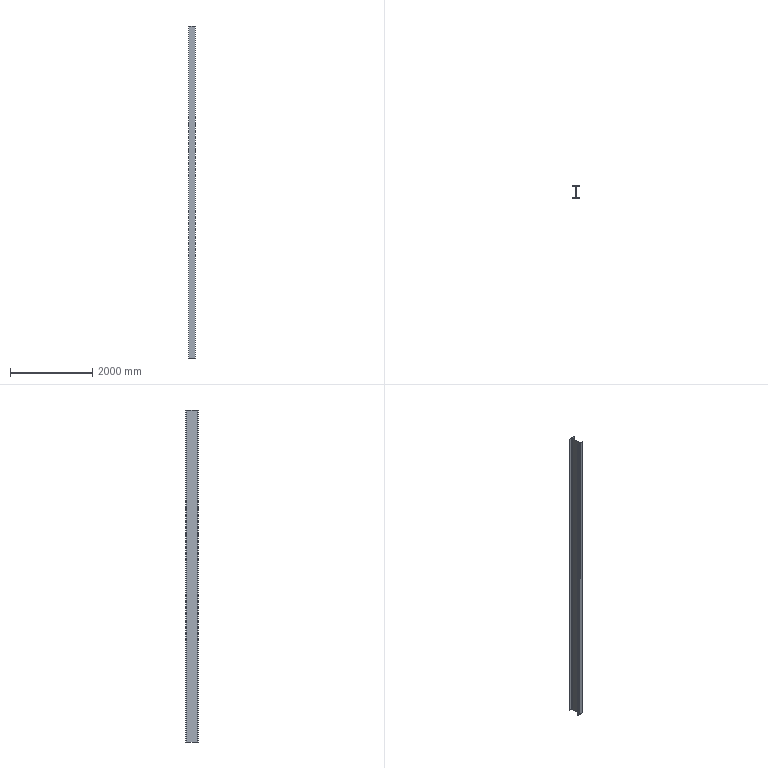Part | SolidWorks | features Extrusion 1 | 1 solid | 18 faces | box 150 x 300 x 8060 mm | volume 37705251 mm3 | plane 14 | cylinder 4 | commonest cylinder face diameters 26 x4
STEP:
#1=CARTESIAN_POINT('',(-75.,9.,0.));
#2=VERTEX_POINT('',#1);
#3=CARTESIAN_POINT('',(-75.,0.,0.));
#4=VERTEX_POINT('',#3);
#5=CARTESIAN_POINT('',(-75.,0.,0.));
#6=DIRECTION('',(0.,-1.,0.));
#7=VECTOR('',#6,1000.);
#8=LINE('',#5,#7);
#9=EDGE_CURVE('',#2,#4,#8,.T.);
#10=ORIENTED_EDGE('',*,*,#9,.T.);
#11=CARTESIAN_POINT('',(-75.,0.,8060.));
#12=VERTEX_POINT('',#11);
#13=CARTESIAN_POINT('',(-75.,0.,8060.));
#14=DIRECTION('',(0.,0.,-1.));
#15=VECTOR('',#14,1000.);
#16=LINE('',#13,#15);
#17=EDGE_CURVE('',#12,#4,#16,.T.);
#18=ORIENTED_EDGE('',*,*,#17,.F.);
#19=CARTESIAN_POINT('',(-75.,9.,8060.));
#20=VERTEX_POINT('',#19);
#21=CARTESIAN_POINT('',(-75.,0.,8060.));
#22=DIRECTION('',(0.,-1.,0.));
#23=VECTOR('',#22,1000.);
#24=LINE('',#21,#23);
#25=EDGE_CURVE('',#20,#12,#24,.T.);
#26=ORIENTED_EDGE('',*,*,#25,.F.);
#27=CARTESIAN_POINT('',(-75.,9.,8060.));
#28=DIRECTION('',(0.,0.,-1.));
#29=VECTOR('',#28,1000.);
#30=LINE('',#27,#29);
#31=EDGE_CURVE('',#20,#2,#30,.T.);
#32=ORIENTED_EDGE('',*,*,#31,.T.);
#33=EDGE_LOOP('',(#10,#18,#26,#32));
#34=FACE_OUTER_BOUND('',#33,.T.);
#35=CARTESIAN_POINT('',(-75.,0.,8060.));
#36=DIRECTION('',(1.,0.,0.));
#37=DIRECTION('',(0.,0.,-1.));
#38=AXIS2_PLACEMENT_3D('',#35,#36,#37);
#39=PLANE('',#38);
#40=ADVANCED_FACE('',(#34),#39,.F.);
#41=CARTESIAN_POINT('',(75.,0.,0.));
#42=VERTEX_POINT('',#41);
#43=CARTESIAN_POINT('',(75.,0.,0.));
#44=DIRECTION('',(1.,0.,0.));
#45=VECTOR('',#44,1000.);
#46=LINE('',#43,#45);
#47=EDGE_CURVE('',#4,#42,#46,.T.);
#48=ORIENTED_EDGE('',*,*,#47,.T.);
#49=CARTESIAN_POINT('',(75.,0.,8060.));
#50=VERTEX_POINT('',#49);
#51=CARTESIAN_POINT('',(75.,0.,8060.));
#52=DIRECTION('',(0.,0.,-1.));
#53=VECTOR('',#52,1000.);
#54=LINE('',#51,#53);
#55=EDGE_CURVE('',#50,#42,#54,.T.);
#56=ORIENTED_EDGE('',*,*,#55,.F.);
#57=CARTESIAN_POINT('',(75.,0.,8060.));
#58=DIRECTION('',(1.,0.,0.));
#59=VECTOR('',#58,1000.);
#60=LINE('',#57,#59);
#61=EDGE_CURVE('',#12,#50,#60,.T.);
#62=ORIENTED_EDGE('',*,*,#61,.F.);
#63=ORIENTED_EDGE('',*,*,#17,.T.);
#64=EDGE_LOOP('',(#48,#56,#62,#63));
#65=FACE_OUTER_BOUND('',#64,.T.);
#66=CARTESIAN_POINT('',(75.,0.,8060.));
#67=DIRECTION('',(0.,1.,0.));
#68=DIRECTION('',(-1.,0.,0.));
#69=AXIS2_PLACEMENT_3D('',#66,#67,#68);
#70=PLANE('',#69);
#71=ADVANCED_FACE('',(#65),#70,.F.);
#72=CARTESIAN_POINT('',(75.,9.,0.));
#73=VERTEX_POINT('',#72);
#74=CARTESIAN_POINT('',(75.,0.,0.));
#75=DIRECTION('',(0.,1.,0.));
#76=VECTOR('',#75,1000.);
#77=LINE('',#74,#76);
#78=EDGE_CURVE('',#42,#73,#77,.T.);
#79=ORIENTED_EDGE('',*,*,#78,.T.);
#80=CARTESIAN_POINT('',(75.,9.,8060.));
#81=VERTEX_POINT('',#80);
#82=CARTESIAN_POINT('',(75.,9.,8060.));
#83=DIRECTION('',(0.,0.,-1.));
#84=VECTOR('',#83,1000.);
#85=LINE('',#82,#84);
#86=EDGE_CURVE('',#81,#73,#85,.T.);
#87=ORIENTED_EDGE('',*,*,#86,.F.);
#88=CARTESIAN_POINT('',(75.,0.,8060.));
#89=DIRECTION('',(0.,1.,0.));
#90=VECTOR('',#89,1000.);
#91=LINE('',#88,#90);
#92=EDGE_CURVE('',#50,#81,#91,.T.);
#93=ORIENTED_EDGE('',*,*,#92,.F.);
#94=ORIENTED_EDGE('',*,*,#55,.T.);
#95=EDGE_LOOP('',(#79,#87,#93,#94));
#96=FACE_OUTER_BOUND('',#95,.T.);
#97=CARTESIAN_POINT('',(75.,0.,8060.));
#98=DIRECTION('',(-1.,0.,0.));
#99=DIRECTION('',(0.,0.,1.));
#100=AXIS2_PLACEMENT_3D('',#97,#98,#99);
#101=PLANE('',#100);
#102=ADVANCED_FACE('',(#96),#101,.F.);
#103=CARTESIAN_POINT('',(16.25,9.,0.));
#104=VERTEX_POINT('',#103);
#105=CARTESIAN_POINT('',(75.,9.,0.));
#106=DIRECTION('',(-1.,0.,0.));
#107=VECTOR('',#106,1000.);
#108=LINE('',#105,#107);
#109=EDGE_CURVE('',#73,#104,#108,.T.);
#110=ORIENTED_EDGE('',*,*,#109,.T.);
#111=CARTESIAN_POINT('',(16.25,9.,8060.));
#112=VERTEX_POINT('',#111);
#113=CARTESIAN_POINT('',(16.25,9.,8060.));
#114=DIRECTION('',(0.,0.,-1.));
#115=VECTOR('',#114,1000.);
#116=LINE('',#113,#115);
#117=EDGE_CURVE('',#112,#104,#116,.T.);
#118=ORIENTED_EDGE('',*,*,#117,.F.);
#119=CARTESIAN_POINT('',(75.,9.,8060.));
#120=DIRECTION('',(-1.,0.,0.));
#121=VECTOR('',#120,1000.);
#122=LINE('',#119,#121);
#123=EDGE_CURVE('',#81,#112,#122,.T.);
#124=ORIENTED_EDGE('',*,*,#123,.F.);
#125=ORIENTED_EDGE('',*,*,#86,.T.);
#126=EDGE_LOOP('',(#110,#118,#124,#125));
#127=FACE_OUTER_BOUND('',#126,.T.);
#128=CARTESIAN_POINT('',(75.,9.,8060.));
#129=DIRECTION('',(0.,-1.,0.));
#130=DIRECTION('',(1.,0.,0.));
#131=AXIS2_PLACEMENT_3D('',#128,#129,#130);
#132=PLANE('',#131);
#133=ADVANCED_FACE('',(#127),#132,.F.);
#134=CARTESIAN_POINT('',(3.25,22.,0.));
#135=VERTEX_POINT('',#134);
#136=CARTESIAN_POINT('',(16.25,22.,0.));
#137=DIRECTION('',(0.,0.,-1.));
#138=DIRECTION('',(-1.,0.,0.));
#139=AXIS2_PLACEMENT_3D('',#136,#137,#138);
#140=CIRCLE('',#139,13.);
#141=EDGE_CURVE('',#104,#135,#140,.T.);
#142=ORIENTED_EDGE('',*,*,#141,.T.);
#143=CARTESIAN_POINT('',(3.25,22.,8060.));
#144=VERTEX_POINT('',#143);
#145=CARTESIAN_POINT('',(3.25,22.,8060.));
#146=DIRECTION('',(0.,0.,-1.));
#147=VECTOR('',#146,1000.);
#148=LINE('',#145,#147);
#149=EDGE_CURVE('',#144,#135,#148,.T.);
#150=ORIENTED_EDGE('',*,*,#149,.F.);
#151=CARTESIAN_POINT('',(16.25,22.,8060.));
#152=DIRECTION('',(0.,0.,-1.));
#153=DIRECTION('',(-1.,0.,0.));
#154=AXIS2_PLACEMENT_3D('',#151,#152,#153);
#155=CIRCLE('',#154,13.);
#156=EDGE_CURVE('',#112,#144,#155,.T.);
#157=ORIENTED_EDGE('',*,*,#156,.F.);
#158=ORIENTED_EDGE('',*,*,#117,.T.);
#159=EDGE_LOOP('',(#142,#150,#157,#158));
#160=FACE_OUTER_BOUND('',#159,.T.);
#161=CARTESIAN_POINT('',(16.25,22.,8060.));
#162=DIRECTION('',(0.,0.,-1.));
#163=DIRECTION('',(-1.,0.,0.));
#164=AXIS2_PLACEMENT_3D('',#161,#162,#163);
#165=CYLINDRICAL_SURFACE('',#164,13.);
#166=ADVANCED_FACE('',(#160),#165,.F.);
#167=CARTESIAN_POINT('',(3.25,278.,0.));
#168=VERTEX_POINT('',#167);
#169=CARTESIAN_POINT('',(3.25,22.,0.));
#170=DIRECTION('',(0.,1.,0.));
#171=VECTOR('',#170,1000.);
#172=LINE('',#169,#171);
#173=EDGE_CURVE('',#135,#168,#172,.T.);
#174=ORIENTED_EDGE('',*,*,#173,.T.);
#175=CARTESIAN_POINT('',(3.25,278.,8060.));
#176=VERTEX_POINT('',#175);
#177=CARTESIAN_POINT('',(3.25,278.,8060.));
#178=DIRECTION('',(0.,0.,-1.));
#179=VECTOR('',#178,1000.);
#180=LINE('',#177,#179);
#181=EDGE_CURVE('',#176,#168,#180,.T.);
#182=ORIENTED_EDGE('',*,*,#181,.F.);
#183=CARTESIAN_POINT('',(3.25,22.,8060.));
#184=DIRECTION('',(0.,1.,0.));
#185=VECTOR('',#184,1000.);
#186=LINE('',#183,#185);
#187=EDGE_CURVE('',#144,#176,#186,.T.);
#188=ORIENTED_EDGE('',*,*,#187,.F.);
#189=ORIENTED_EDGE('',*,*,#149,.T.);
#190=EDGE_LOOP('',(#174,#182,#188,#189));
#191=FACE_OUTER_BOUND('',#190,.T.);
#192=CARTESIAN_POINT('',(3.25,22.,8060.));
#193=DIRECTION('',(-1.,0.,0.));
#194=DIRECTION('',(0.,0.,1.));
#195=AXIS2_PLACEMENT_3D('',#192,#193,#194);
#196=PLANE('',#195);
#197=ADVANCED_FACE('',(#191),#196,.F.);
#198=CARTESIAN_POINT('',(16.25,291.,0.));
#199=VERTEX_POINT('',#198);
#200=CARTESIAN_POINT('',(16.25,278.,0.));
#201=DIRECTION('',(0.,0.,-1.));
#202=DIRECTION('',(-1.,0.,0.));
#203=AXIS2_PLACEMENT_3D('',#200,#201,#202);
#204=CIRCLE('',#203,13.);
#205=EDGE_CURVE('',#168,#199,#204,.T.);
#206=ORIENTED_EDGE('',*,*,#205,.T.);
#207=CARTESIAN_POINT('',(16.25,291.,8060.));
#208=VERTEX_POINT('',#207);
#209=CARTESIAN_POINT('',(16.25,291.,8060.));
#210=DIRECTION('',(0.,0.,-1.));
#211=VECTOR('',#210,1000.);
#212=LINE('',#209,#211);
#213=EDGE_CURVE('',#208,#199,#212,.T.);
#214=ORIENTED_EDGE('',*,*,#213,.F.);
#215=CARTESIAN_POINT('',(16.25,278.,8060.));
#216=DIRECTION('',(0.,0.,-1.));
#217=DIRECTION('',(-1.,0.,0.));
#218=AXIS2_PLACEMENT_3D('',#215,#216,#217);
#219=CIRCLE('',#218,13.);
#220=EDGE_CURVE('',#176,#208,#219,.T.);
#221=ORIENTED_EDGE('',*,*,#220,.F.);
#222=ORIENTED_EDGE('',*,*,#181,.T.);
#223=EDGE_LOOP('',(#206,#214,#221,#222));
#224=FACE_OUTER_BOUND('',#223,.T.);
#225=CARTESIAN_POINT('',(16.25,278.,8060.));
#226=DIRECTION('',(0.,0.,-1.));
#227=DIRECTION('',(-1.,0.,0.));
#228=AXIS2_PLACEMENT_3D('',#225,#226,#227);
#229=CYLINDRICAL_SURFACE('',#228,13.);
#230=ADVANCED_FACE('',(#224),#229,.F.);
#231=CARTESIAN_POINT('',(75.,291.,0.));
#232=VERTEX_POINT('',#231);
#233=CARTESIAN_POINT('',(16.25,291.,0.));
#234=DIRECTION('',(1.,0.,0.));
#235=VECTOR('',#234,1000.);
#236=LINE('',#233,#235);
#237=EDGE_CURVE('',#199,#232,#236,.T.);
#238=ORIENTED_EDGE('',*,*,#237,.T.);
#239=CARTESIAN_POINT('',(75.,291.,8060.));
#240=VERTEX_POINT('',#239);
#241=CARTESIAN_POINT('',(75.,291.,8060.));
#242=DIRECTION('',(0.,0.,-1.));
#243=VECTOR('',#242,1000.);
#244=LINE('',#241,#243);
#245=EDGE_CURVE('',#240,#232,#244,.T.);
#246=ORIENTED_EDGE('',*,*,#245,.F.);
#247=CARTESIAN_POINT('',(16.25,291.,8060.));
#248=DIRECTION('',(1.,0.,0.));
#249=VECTOR('',#248,1000.);
#250=LINE('',#247,#249);
#251=EDGE_CURVE('',#208,#240,#250,.T.);
#252=ORIENTED_EDGE('',*,*,#251,.F.);
#253=ORIENTED_EDGE('',*,*,#213,.T.);
#254=EDGE_LOOP('',(#238,#246,#252,#253));
#255=FACE_OUTER_BOUND('',#254,.T.);
#256=CARTESIAN_POINT('',(16.25,291.,8060.));
#257=DIRECTION('',(0.,1.,0.));
#258=DIRECTION('',(-1.,0.,0.));
#259=AXIS2_PLACEMENT_3D('',#256,#257,#258);
#260=PLANE('',#259);
#261=ADVANCED_FACE('',(#255),#260,.F.);
#262=CARTESIAN_POINT('',(75.,300.,0.));
#263=VERTEX_POINT('',#262);
#264=CARTESIAN_POINT('',(75.,291.,0.));
#265=DIRECTION('',(0.,1.,0.));
#266=VECTOR('',#265,1000.);
#267=LINE('',#264,#266);
#268=EDGE_CURVE('',#232,#263,#267,.T.);
#269=ORIENTED_EDGE('',*,*,#268,.T.);
#270=CARTESIAN_POINT('',(75.,300.,8060.));
#271=VERTEX_POINT('',#270);
#272=CARTESIAN_POINT('',(75.,300.,8060.));
#273=DIRECTION('',(0.,0.,-1.));
#274=VECTOR('',#273,1000.);
#275=LINE('',#272,#274);
#276=EDGE_CURVE('',#271,#263,#275,.T.);
#277=ORIENTED_EDGE('',*,*,#276,.F.);
#278=CARTESIAN_POINT('',(75.,291.,8060.));
#279=DIRECTION('',(0.,1.,0.));
#280=VECTOR('',#279,1000.);
#281=LINE('',#278,#280);
#282=EDGE_CURVE('',#240,#271,#281,.T.);
#283=ORIENTED_EDGE('',*,*,#282,.F.);
#284=ORIENTED_EDGE('',*,*,#245,.T.);
#285=EDGE_LOOP('',(#269,#277,#283,#284));
#286=FACE_OUTER_BOUND('',#285,.T.);
#287=CARTESIAN_POINT('',(75.,291.,8060.));
#288=DIRECTION('',(-1.,0.,0.));
#289=DIRECTION('',(0.,-1.,0.));
#290=AXIS2_PLACEMENT_3D('',#287,#288,#289);
#291=PLANE('',#290);
#292=ADVANCED_FACE('',(#286),#291,.F.);
#293=CARTESIAN_POINT('',(-75.,300.,0.));
#294=VERTEX_POINT('',#293);
#295=CARTESIAN_POINT('',(-75.,300.,0.));
#296=DIRECTION('',(-1.,0.,0.));
#297=VECTOR('',#296,1000.);
#298=LINE('',#295,#297);
#299=EDGE_CURVE('',#263,#294,#298,.T.);
#300=ORIENTED_EDGE('',*,*,#299,.T.);
#301=CARTESIAN_POINT('',(-75.,300.,8060.));
#302=VERTEX_POINT('',#301);
#303=CARTESIAN_POINT('',(-75.,300.,8060.));
#304=DIRECTION('',(0.,0.,-1.));
#305=VECTOR('',#304,1000.);
#306=LINE('',#303,#305);
#307=EDGE_CURVE('',#302,#294,#306,.T.);
#308=ORIENTED_EDGE('',*,*,#307,.F.);
#309=CARTESIAN_POINT('',(-75.,300.,8060.));
#310=DIRECTION('',(-1.,0.,0.));
#311=VECTOR('',#310,1000.);
#312=LINE('',#309,#311);
#313=EDGE_CURVE('',#271,#302,#312,.T.);
#314=ORIENTED_EDGE('',*,*,#313,.F.);
#315=ORIENTED_EDGE('',*,*,#276,.T.);
#316=EDGE_LOOP('',(#300,#308,#314,#315));
#317=FACE_OUTER_BOUND('',#316,.T.);
#318=CARTESIAN_POINT('',(-75.,300.,8060.));
#319=DIRECTION('',(0.,-1.,0.));
#320=DIRECTION('',(0.,0.,-1.));
#321=AXIS2_PLACEMENT_3D('',#318,#319,#320);
#322=PLANE('',#321);
#323=ADVANCED_FACE('',(#317),#322,.F.);
#324=CARTESIAN_POINT('',(-75.,291.,0.));
#325=VERTEX_POINT('',#324);
#326=CARTESIAN_POINT('',(-75.,291.,0.));
#327=DIRECTION('',(0.,-1.,0.));
#328=VECTOR('',#327,1000.);
#329=LINE('',#326,#328);
#330=EDGE_CURVE('',#294,#325,#329,.T.);
#331=ORIENTED_EDGE('',*,*,#330,.T.);
#332=CARTESIAN_POINT('',(-75.,291.,8060.));
#333=VERTEX_POINT('',#332);
#334=CARTESIAN_POINT('',(-75.,291.,8060.));
#335=DIRECTION('',(0.,0.,-1.));
#336=VECTOR('',#335,1000.);
#337=LINE('',#334,#336);
#338=EDGE_CURVE('',#333,#325,#337,.T.);
#339=ORIENTED_EDGE('',*,*,#338,.F.);
#340=CARTESIAN_POINT('',(-75.,291.,8060.));
#341=DIRECTION('',(0.,-1.,0.));
#342=VECTOR('',#341,1000.);
#343=LINE('',#340,#342);
#344=EDGE_CURVE('',#302,#333,#343,.T.);
#345=ORIENTED_EDGE('',*,*,#344,.F.);
#346=ORIENTED_EDGE('',*,*,#307,.T.);
#347=EDGE_LOOP('',(#331,#339,#345,#346));
#348=FACE_OUTER_BOUND('',#347,.T.);
#349=CARTESIAN_POINT('',(-75.,291.,8060.));
#350=DIRECTION('',(1.,0.,0.));
#351=DIRECTION('',(0.,1.,0.));
#352=AXIS2_PLACEMENT_3D('',#349,#350,#351);
#353=PLANE('',#352);
#354=ADVANCED_FACE('',(#348),#353,.F.);
#355=CARTESIAN_POINT('',(-16.25,291.,0.));
#356=VERTEX_POINT('',#355);
#357=CARTESIAN_POINT('',(-16.25,291.,0.));
#358=DIRECTION('',(1.,0.,0.));
#359=VECTOR('',#358,1000.);
#360=LINE('',#357,#359);
#361=EDGE_CURVE('',#325,#356,#360,.T.);
#362=ORIENTED_EDGE('',*,*,#361,.T.);
#363=CARTESIAN_POINT('',(-16.25,291.,8060.));
#364=VERTEX_POINT('',#363);
#365=CARTESIAN_POINT('',(-16.25,291.,8060.));
#366=DIRECTION('',(0.,0.,-1.));
#367=VECTOR('',#366,1000.);
#368=LINE('',#365,#367);
#369=EDGE_CURVE('',#364,#356,#368,.T.);
#370=ORIENTED_EDGE('',*,*,#369,.F.);
#371=CARTESIAN_POINT('',(-16.25,291.,8060.));
#372=DIRECTION('',(1.,0.,0.));
#373=VECTOR('',#372,1000.);
#374=LINE('',#371,#373);
#375=EDGE_CURVE('',#333,#364,#374,.T.);
#376=ORIENTED_EDGE('',*,*,#375,.F.);
#377=ORIENTED_EDGE('',*,*,#338,.T.);
#378=EDGE_LOOP('',(#362,#370,#376,#377));
#379=FACE_OUTER_BOUND('',#378,.T.);
#380=CARTESIAN_POINT('',(-16.25,291.,8060.));
#381=DIRECTION('',(0.,1.,0.));
#382=DIRECTION('',(-1.,0.,0.));
#383=AXIS2_PLACEMENT_3D('',#380,#381,#382);
#384=PLANE('',#383);
#385=ADVANCED_FACE('',(#379),#384,.F.);
#386=CARTESIAN_POINT('',(-3.25,278.,0.));
#387=VERTEX_POINT('',#386);
#388=CARTESIAN_POINT('',(-16.25,278.,0.));
#389=DIRECTION('',(0.,0.,-1.));
#390=DIRECTION('',(1.,0.,0.));
#391=AXIS2_PLACEMENT_3D('',#388,#389,#390);
#392=CIRCLE('',#391,13.);
#393=EDGE_CURVE('',#356,#387,#392,.T.);
#394=ORIENTED_EDGE('',*,*,#393,.T.);
#395=CARTESIAN_POINT('',(-3.25,278.,8060.));
#396=VERTEX_POINT('',#395);
#397=CARTESIAN_POINT('',(-3.25,278.,8060.));
#398=DIRECTION('',(0.,0.,-1.));
#399=VECTOR('',#398,1000.);
#400=LINE('',#397,#399);
#401=EDGE_CURVE('',#396,#387,#400,.T.);
#402=ORIENTED_EDGE('',*,*,#401,.F.);
#403=CARTESIAN_POINT('',(-16.25,278.,8060.));
#404=DIRECTION('',(0.,0.,-1.));
#405=DIRECTION('',(1.,0.,0.));
#406=AXIS2_PLACEMENT_3D('',#403,#404,#405);
#407=CIRCLE('',#406,13.);
#408=EDGE_CURVE('',#364,#396,#407,.T.);
#409=ORIENTED_EDGE('',*,*,#408,.F.);
#410=ORIENTED_EDGE('',*,*,#369,.T.);
#411=EDGE_LOOP('',(#394,#402,#409,#410));
#412=FACE_OUTER_BOUND('',#411,.T.);
#413=CARTESIAN_POINT('',(-16.25,278.,8060.));
#414=DIRECTION('',(0.,0.,-1.));
#415=DIRECTION('',(-1.,0.,0.));
#416=AXIS2_PLACEMENT_3D('',#413,#414,#415);
#417=CYLINDRICAL_SURFACE('',#416,13.);
#418=ADVANCED_FACE('',(#412),#417,.F.);
#419=CARTESIAN_POINT('',(-3.25,22.,0.));
#420=VERTEX_POINT('',#419);
#421=CARTESIAN_POINT('',(-3.25,22.,0.));
#422=DIRECTION('',(0.,-1.,0.));
#423=VECTOR('',#422,1000.);
#424=LINE('',#421,#423);
#425=EDGE_CURVE('',#387,#420,#424,.T.);
#426=ORIENTED_EDGE('',*,*,#425,.T.);
#427=CARTESIAN_POINT('',(-3.25,22.,8060.));
#428=VERTEX_POINT('',#427);
#429=CARTESIAN_POINT('',(-3.25,22.,8060.));
#430=DIRECTION('',(0.,0.,-1.));
#431=VECTOR('',#430,1000.);
#432=LINE('',#429,#431);
#433=EDGE_CURVE('',#428,#420,#432,.T.);
#434=ORIENTED_EDGE('',*,*,#433,.F.);
#435=CARTESIAN_POINT('',(-3.25,22.,8060.));
#436=DIRECTION('',(0.,-1.,0.));
#437=VECTOR('',#436,1000.);
#438=LINE('',#435,#437);
#439=EDGE_CURVE('',#396,#428,#438,.T.);
#440=ORIENTED_EDGE('',*,*,#439,.F.);
#441=ORIENTED_EDGE('',*,*,#401,.T.);
#442=EDGE_LOOP('',(#426,#434,#440,#441));
#443=FACE_OUTER_BOUND('',#442,.T.);
#444=CARTESIAN_POINT('',(-3.25,22.,8060.));
#445=DIRECTION('',(1.,0.,0.));
#446=DIRECTION('',(0.,0.,-1.));
#447=AXIS2_PLACEMENT_3D('',#444,#445,#446);
#448=PLANE('',#447);
#449=ADVANCED_FACE('',(#443),#448,.F.);
#450=CARTESIAN_POINT('',(-16.25,9.,0.));
#451=VERTEX_POINT('',#450);
#452=CARTESIAN_POINT('',(-16.25,22.,0.));
#453=DIRECTION('',(0.,0.,-1.));
#454=DIRECTION('',(-1.,0.,0.));
#455=AXIS2_PLACEMENT_3D('',#452,#453,#454);
#456=CIRCLE('',#455,13.);
#457=EDGE_CURVE('',#420,#451,#456,.T.);
#458=ORIENTED_EDGE('',*,*,#457,.T.);
#459=CARTESIAN_POINT('',(-16.25,9.,8060.));
#460=VERTEX_POINT('',#459);
#461=CARTESIAN_POINT('',(-16.25,9.,8060.));
#462=DIRECTION('',(0.,0.,-1.));
#463=VECTOR('',#462,1000.);
#464=LINE('',#461,#463);
#465=EDGE_CURVE('',#460,#451,#464,.T.);
#466=ORIENTED_EDGE('',*,*,#465,.F.);
#467=CARTESIAN_POINT('',(-16.25,22.,8060.));
#468=DIRECTION('',(0.,0.,-1.));
#469=DIRECTION('',(-1.,0.,0.));
#470=AXIS2_PLACEMENT_3D('',#467,#468,#469);
#471=CIRCLE('',#470,13.);
#472=EDGE_CURVE('',#428,#460,#471,.T.);
#473=ORIENTED_EDGE('',*,*,#472,.F.);
#474=ORIENTED_EDGE('',*,*,#433,.T.);
#475=EDGE_LOOP('',(#458,#466,#473,#474));
#476=FACE_OUTER_BOUND('',#475,.T.);
#477=CARTESIAN_POINT('',(-16.25,22.,8060.));
#478=DIRECTION('',(0.,0.,-1.));
#479=DIRECTION('',(-1.,0.,0.));
#480=AXIS2_PLACEMENT_3D('',#477,#478,#479);
#481=CYLINDRICAL_SURFACE('',#480,13.);
#482=ADVANCED_FACE('',(#476),#481,.F.);
#483=CARTESIAN_POINT('',(-75.,9.,0.));
#484=DIRECTION('',(-1.,0.,0.));
#485=VECTOR('',#484,1000.);
#486=LINE('',#483,#485);
#487=EDGE_CURVE('',#451,#2,#486,.T.);
#488=ORIENTED_EDGE('',*,*,#487,.T.);
#489=ORIENTED_EDGE('',*,*,#31,.F.);
#490=CARTESIAN_POINT('',(-75.,9.,8060.));
#491=DIRECTION('',(-1.,0.,0.));
#492=VECTOR('',#491,1000.);
#493=LINE('',#490,#492);
#494=EDGE_CURVE('',#460,#20,#493,.T.);
#495=ORIENTED_EDGE('',*,*,#494,.F.);
#496=ORIENTED_EDGE('',*,*,#465,.T.);
#497=EDGE_LOOP('',(#488,#489,#495,#496));
#498=FACE_OUTER_BOUND('',#497,.T.);
#499=CARTESIAN_POINT('',(-75.,9.,8060.));
#500=DIRECTION('',(0.,-1.,0.));
#501=DIRECTION('',(1.,0.,0.));
#502=AXIS2_PLACEMENT_3D('',#499,#500,#501);
#503=PLANE('',#502);
#504=ADVANCED_FACE('',(#498),#503,.F.);
#505=ORIENTED_EDGE('',*,*,#25,.T.);
#506=ORIENTED_EDGE('',*,*,#61,.T.);
#507=ORIENTED_EDGE('',*,*,#92,.T.);
#508=ORIENTED_EDGE('',*,*,#123,.T.);
#509=ORIENTED_EDGE('',*,*,#156,.T.);
#510=ORIENTED_EDGE('',*,*,#187,.T.);
#511=ORIENTED_EDGE('',*,*,#220,.T.);
#512=ORIENTED_EDGE('',*,*,#251,.T.);
#513=ORIENTED_EDGE('',*,*,#282,.T.);
#514=ORIENTED_EDGE('',*,*,#313,.T.);
#515=ORIENTED_EDGE('',*,*,#344,.T.);
#516=ORIENTED_EDGE('',*,*,#375,.T.);
#517=ORIENTED_EDGE('',*,*,#408,.T.);
#518=ORIENTED_EDGE('',*,*,#439,.T.);
#519=ORIENTED_EDGE('',*,*,#472,.T.);
#520=ORIENTED_EDGE('',*,*,#494,.T.);
#521=EDGE_LOOP('',(#505,#506,#507,#508,#509,#510,#511,#512,#513,#514,#515,#516,#517,#518,#519,#520));
#522=FACE_OUTER_BOUND('',#521,.T.);
#523=CARTESIAN_POINT('',(-16.25,22.,8060.));
#524=DIRECTION('',(0.,0.,-1.));
#525=DIRECTION('',(-1.,0.,0.));
#526=AXIS2_PLACEMENT_3D('',#523,#524,#525);
#527=PLANE('',#526);
#528=ADVANCED_FACE('',(#522),#527,.F.);
#529=ORIENTED_EDGE('',*,*,#9,.F.);
#530=ORIENTED_EDGE('',*,*,#487,.F.);
#531=ORIENTED_EDGE('',*,*,#457,.F.);
#532=ORIENTED_EDGE('',*,*,#425,.F.);
#533=ORIENTED_EDGE('',*,*,#393,.F.);
#534=ORIENTED_EDGE('',*,*,#361,.F.);
#535=ORIENTED_EDGE('',*,*,#330,.F.);
#536=ORIENTED_EDGE('',*,*,#299,.F.);
#537=ORIENTED_EDGE('',*,*,#268,.F.);
#538=ORIENTED_EDGE('',*,*,#237,.F.);
#539=ORIENTED_EDGE('',*,*,#205,.F.);
#540=ORIENTED_EDGE('',*,*,#173,.F.);
#541=ORIENTED_EDGE('',*,*,#141,.F.);
#542=ORIENTED_EDGE('',*,*,#109,.F.);
#543=ORIENTED_EDGE('',*,*,#78,.F.);
#544=ORIENTED_EDGE('',*,*,#47,.F.);
#545=EDGE_LOOP('',(#529,#530,#531,#532,#533,#534,#535,#536,#537,#538,#539,#540,#541,#542,#543,#544));
#546=FACE_OUTER_BOUND('',#545,.T.);
#547=CARTESIAN_POINT('',(-16.25,22.,0.));
#548=DIRECTION('',(0.,0.,-1.));
#549=DIRECTION('',(-1.,0.,0.));
#550=AXIS2_PLACEMENT_3D('',#547,#548,#549);
#551=PLANE('',#550);
#552=ADVANCED_FACE('',(#546),#551,.T.);
#553=CLOSED_SHELL('',(#40,#71,#102,#133,#166,#197,#230,#261,#292,#323,#354,#385,#418,#449,#482,#504,#528,#552));
#554=MANIFOLD_SOLID_BREP('',#553);
#555=CARTESIAN_POINT('',(0.,0.,0.));
#556=DIRECTION('',(0.,0.,1.));
#557=DIRECTION('',(1.,0.,0.));
#558=AXIS2_PLACEMENT_3D('',#555,#556,#557);
#559=(LENGTH_UNIT()NAMED_UNIT(*)SI_UNIT(.MILLI.,.METRE.));
#560=UNCERTAINTY_MEASURE_WITH_UNIT(LENGTH_MEASURE(0.00001),#559,'','');
#561=(NAMED_UNIT(*)PLANE_ANGLE_UNIT()SI_UNIT($,.RADIAN.));
#562=(NAMED_UNIT(*)SI_UNIT($,.STERADIAN.)SOLID_ANGLE_UNIT());
#563=(GEOMETRIC_REPRESENTATION_CONTEXT(3)GLOBAL_UNCERTAINTY_ASSIGNED_CONTEXT((#560))GLOBAL_UNIT_ASSIGNED_CONTEXT((#559,#561,#562))REPRESENTATION_CONTEXT('',''));
#564=ADVANCED_BREP_SHAPE_REPRESENTATION('',(#554,#558),#563);